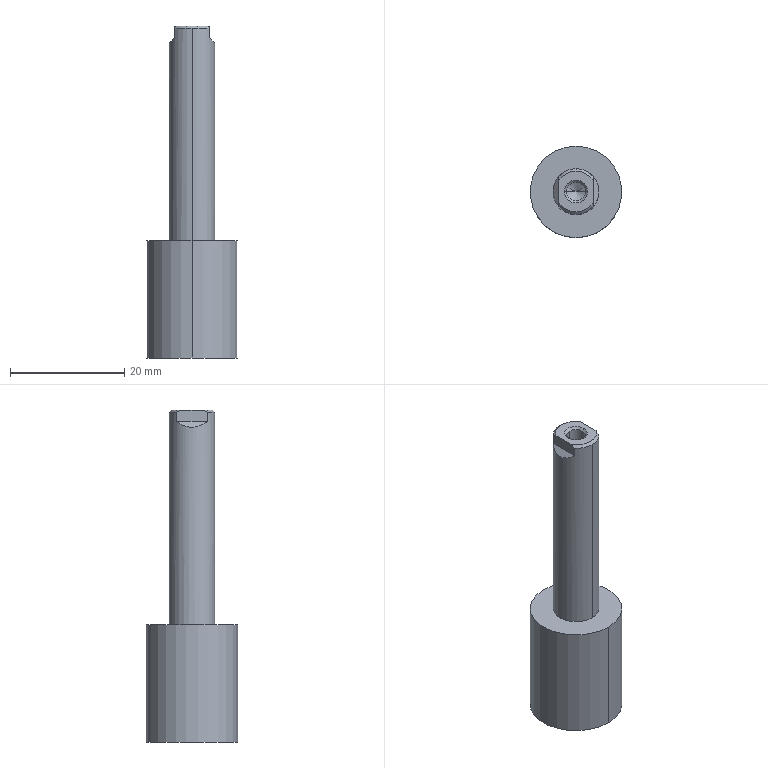Part | STEP file | HI_JSNR16X30_rod_default | 1 solid | 20 faces | box 16 x 16 x 58 mm | volume 5910 mm3 | cone 7 | plane 7 | cylinder 6 | commonest cylinder face diameters 3.242 x2 8 x2 16 x2